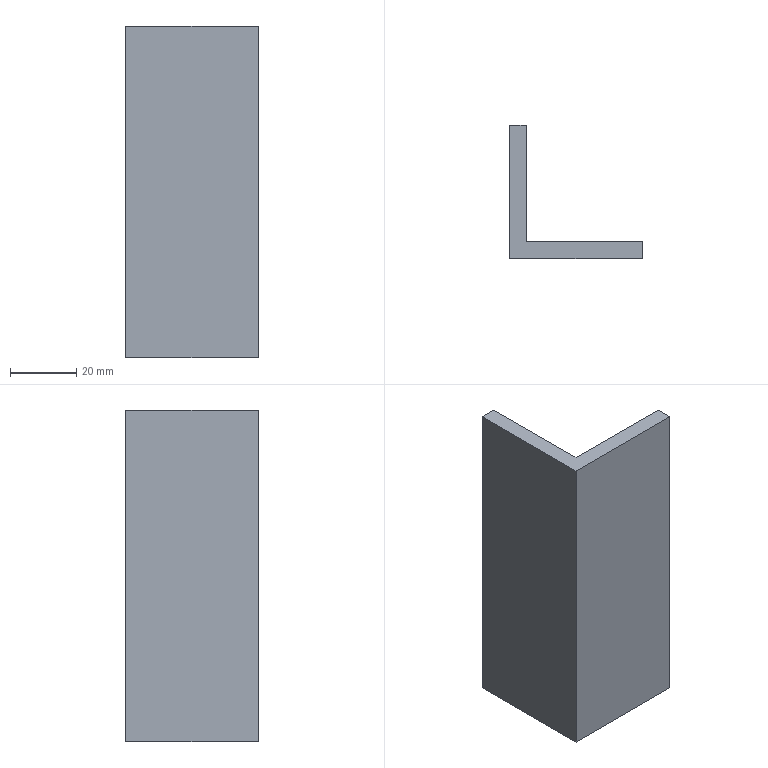Part | SolidWorks | features Extrusion 1 | 1 solid | 8 faces | box 40 x 40 x 100 mm | volume 37500 mm3 | plane 8
STEP:
#1=CARTESIAN_POINT('',(5.,0.,0.));
#2=VERTEX_POINT('',#1);
#3=CARTESIAN_POINT('',(0.,0.,0.));
#4=VERTEX_POINT('',#3);
#5=CARTESIAN_POINT('',(0.,0.,0.));
#6=DIRECTION('',(-1.,0.,0.));
#7=VECTOR('',#6,1000.);
#8=LINE('',#5,#7);
#9=EDGE_CURVE('',#2,#4,#8,.T.);
#10=ORIENTED_EDGE('',*,*,#9,.T.);
#11=CARTESIAN_POINT('',(0.,0.,100.));
#12=VERTEX_POINT('',#11);
#13=CARTESIAN_POINT('',(0.,0.,100.));
#14=DIRECTION('',(0.,0.,-1.));
#15=VECTOR('',#14,1000.);
#16=LINE('',#13,#15);
#17=EDGE_CURVE('',#12,#4,#16,.T.);
#18=ORIENTED_EDGE('',*,*,#17,.F.);
#19=CARTESIAN_POINT('',(5.,0.,100.));
#20=VERTEX_POINT('',#19);
#21=CARTESIAN_POINT('',(0.,0.,100.));
#22=DIRECTION('',(-1.,0.,0.));
#23=VECTOR('',#22,1000.);
#24=LINE('',#21,#23);
#25=EDGE_CURVE('',#20,#12,#24,.T.);
#26=ORIENTED_EDGE('',*,*,#25,.F.);
#27=CARTESIAN_POINT('',(5.,0.,100.));
#28=DIRECTION('',(0.,0.,-1.));
#29=VECTOR('',#28,1000.);
#30=LINE('',#27,#29);
#31=EDGE_CURVE('',#20,#2,#30,.T.);
#32=ORIENTED_EDGE('',*,*,#31,.T.);
#33=EDGE_LOOP('',(#10,#18,#26,#32));
#34=FACE_OUTER_BOUND('',#33,.T.);
#35=CARTESIAN_POINT('',(0.,0.,100.));
#36=DIRECTION('',(0.,-1.,0.));
#37=DIRECTION('',(0.,0.,-1.));
#38=AXIS2_PLACEMENT_3D('',#35,#36,#37);
#39=PLANE('',#38);
#40=ADVANCED_FACE('',(#34),#39,.F.);
#41=CARTESIAN_POINT('',(0.,-40.,0.));
#42=VERTEX_POINT('',#41);
#43=CARTESIAN_POINT('',(0.,0.,0.));
#44=DIRECTION('',(0.,-1.,0.));
#45=VECTOR('',#44,1000.);
#46=LINE('',#43,#45);
#47=EDGE_CURVE('',#4,#42,#46,.T.);
#48=ORIENTED_EDGE('',*,*,#47,.T.);
#49=CARTESIAN_POINT('',(0.,-40.,100.));
#50=VERTEX_POINT('',#49);
#51=CARTESIAN_POINT('',(0.,-40.,100.));
#52=DIRECTION('',(0.,0.,-1.));
#53=VECTOR('',#52,1000.);
#54=LINE('',#51,#53);
#55=EDGE_CURVE('',#50,#42,#54,.T.);
#56=ORIENTED_EDGE('',*,*,#55,.F.);
#57=CARTESIAN_POINT('',(0.,0.,100.));
#58=DIRECTION('',(0.,-1.,0.));
#59=VECTOR('',#58,1000.);
#60=LINE('',#57,#59);
#61=EDGE_CURVE('',#12,#50,#60,.T.);
#62=ORIENTED_EDGE('',*,*,#61,.F.);
#63=ORIENTED_EDGE('',*,*,#17,.T.);
#64=EDGE_LOOP('',(#48,#56,#62,#63));
#65=FACE_OUTER_BOUND('',#64,.T.);
#66=CARTESIAN_POINT('',(0.,0.,100.));
#67=DIRECTION('',(1.,0.,0.));
#68=DIRECTION('',(0.,1.,0.));
#69=AXIS2_PLACEMENT_3D('',#66,#67,#68);
#70=PLANE('',#69);
#71=ADVANCED_FACE('',(#65),#70,.F.);
#72=CARTESIAN_POINT('',(40.,-40.,0.));
#73=VERTEX_POINT('',#72);
#74=CARTESIAN_POINT('',(0.,-40.,0.));
#75=DIRECTION('',(1.,0.,0.));
#76=VECTOR('',#75,1000.);
#77=LINE('',#74,#76);
#78=EDGE_CURVE('',#42,#73,#77,.T.);
#79=ORIENTED_EDGE('',*,*,#78,.T.);
#80=CARTESIAN_POINT('',(40.,-40.,100.));
#81=VERTEX_POINT('',#80);
#82=CARTESIAN_POINT('',(40.,-40.,100.));
#83=DIRECTION('',(0.,0.,-1.));
#84=VECTOR('',#83,1000.);
#85=LINE('',#82,#84);
#86=EDGE_CURVE('',#81,#73,#85,.T.);
#87=ORIENTED_EDGE('',*,*,#86,.F.);
#88=CARTESIAN_POINT('',(0.,-40.,100.));
#89=DIRECTION('',(1.,0.,0.));
#90=VECTOR('',#89,1000.);
#91=LINE('',#88,#90);
#92=EDGE_CURVE('',#50,#81,#91,.T.);
#93=ORIENTED_EDGE('',*,*,#92,.F.);
#94=ORIENTED_EDGE('',*,*,#55,.T.);
#95=EDGE_LOOP('',(#79,#87,#93,#94));
#96=FACE_OUTER_BOUND('',#95,.T.);
#97=CARTESIAN_POINT('',(0.,-40.,100.));
#98=DIRECTION('',(0.,1.,0.));
#99=DIRECTION('',(0.,0.,1.));
#100=AXIS2_PLACEMENT_3D('',#97,#98,#99);
#101=PLANE('',#100);
#102=ADVANCED_FACE('',(#96),#101,.F.);
#103=CARTESIAN_POINT('',(40.,-35.,0.));
#104=VERTEX_POINT('',#103);
#105=CARTESIAN_POINT('',(40.,-40.,0.));
#106=DIRECTION('',(0.,1.,0.));
#107=VECTOR('',#106,1000.);
#108=LINE('',#105,#107);
#109=EDGE_CURVE('',#73,#104,#108,.T.);
#110=ORIENTED_EDGE('',*,*,#109,.T.);
#111=CARTESIAN_POINT('',(40.,-35.,100.));
#112=VERTEX_POINT('',#111);
#113=CARTESIAN_POINT('',(40.,-35.,100.));
#114=DIRECTION('',(0.,0.,-1.));
#115=VECTOR('',#114,1000.);
#116=LINE('',#113,#115);
#117=EDGE_CURVE('',#112,#104,#116,.T.);
#118=ORIENTED_EDGE('',*,*,#117,.F.);
#119=CARTESIAN_POINT('',(40.,-40.,100.));
#120=DIRECTION('',(0.,1.,0.));
#121=VECTOR('',#120,1000.);
#122=LINE('',#119,#121);
#123=EDGE_CURVE('',#81,#112,#122,.T.);
#124=ORIENTED_EDGE('',*,*,#123,.F.);
#125=ORIENTED_EDGE('',*,*,#86,.T.);
#126=EDGE_LOOP('',(#110,#118,#124,#125));
#127=FACE_OUTER_BOUND('',#126,.T.);
#128=CARTESIAN_POINT('',(40.,-40.,100.));
#129=DIRECTION('',(-1.,0.,0.));
#130=DIRECTION('',(0.,0.,1.));
#131=AXIS2_PLACEMENT_3D('',#128,#129,#130);
#132=PLANE('',#131);
#133=ADVANCED_FACE('',(#127),#132,.F.);
#134=CARTESIAN_POINT('',(5.,-35.,0.));
#135=VERTEX_POINT('',#134);
#136=CARTESIAN_POINT('',(5.,-35.,0.));
#137=DIRECTION('',(-1.,0.,0.));
#138=VECTOR('',#137,1000.);
#139=LINE('',#136,#138);
#140=EDGE_CURVE('',#104,#135,#139,.T.);
#141=ORIENTED_EDGE('',*,*,#140,.T.);
#142=CARTESIAN_POINT('',(5.,-35.,100.));
#143=VERTEX_POINT('',#142);
#144=CARTESIAN_POINT('',(5.,-35.,100.));
#145=DIRECTION('',(0.,0.,-1.));
#146=VECTOR('',#145,1000.);
#147=LINE('',#144,#146);
#148=EDGE_CURVE('',#143,#135,#147,.T.);
#149=ORIENTED_EDGE('',*,*,#148,.F.);
#150=CARTESIAN_POINT('',(5.,-35.,100.));
#151=DIRECTION('',(-1.,0.,0.));
#152=VECTOR('',#151,1000.);
#153=LINE('',#150,#152);
#154=EDGE_CURVE('',#112,#143,#153,.T.);
#155=ORIENTED_EDGE('',*,*,#154,.F.);
#156=ORIENTED_EDGE('',*,*,#117,.T.);
#157=EDGE_LOOP('',(#141,#149,#155,#156));
#158=FACE_OUTER_BOUND('',#157,.T.);
#159=CARTESIAN_POINT('',(5.,-35.,100.));
#160=DIRECTION('',(0.,-1.,0.));
#161=DIRECTION('',(0.,0.,-1.));
#162=AXIS2_PLACEMENT_3D('',#159,#160,#161);
#163=PLANE('',#162);
#164=ADVANCED_FACE('',(#158),#163,.F.);
#165=CARTESIAN_POINT('',(5.,0.,0.));
#166=DIRECTION('',(0.,1.,0.));
#167=VECTOR('',#166,1000.);
#168=LINE('',#165,#167);
#169=EDGE_CURVE('',#135,#2,#168,.T.);
#170=ORIENTED_EDGE('',*,*,#169,.T.);
#171=ORIENTED_EDGE('',*,*,#31,.F.);
#172=CARTESIAN_POINT('',(5.,0.,100.));
#173=DIRECTION('',(0.,1.,0.));
#174=VECTOR('',#173,1000.);
#175=LINE('',#172,#174);
#176=EDGE_CURVE('',#143,#20,#175,.T.);
#177=ORIENTED_EDGE('',*,*,#176,.F.);
#178=ORIENTED_EDGE('',*,*,#148,.T.);
#179=EDGE_LOOP('',(#170,#171,#177,#178));
#180=FACE_OUTER_BOUND('',#179,.T.);
#181=CARTESIAN_POINT('',(5.,0.,100.));
#182=DIRECTION('',(-1.,0.,0.));
#183=DIRECTION('',(0.,0.,1.));
#184=AXIS2_PLACEMENT_3D('',#181,#182,#183);
#185=PLANE('',#184);
#186=ADVANCED_FACE('',(#180),#185,.F.);
#187=ORIENTED_EDGE('',*,*,#25,.T.);
#188=ORIENTED_EDGE('',*,*,#61,.T.);
#189=ORIENTED_EDGE('',*,*,#92,.T.);
#190=ORIENTED_EDGE('',*,*,#123,.T.);
#191=ORIENTED_EDGE('',*,*,#154,.T.);
#192=ORIENTED_EDGE('',*,*,#176,.T.);
#193=EDGE_LOOP('',(#187,#188,#189,#190,#191,#192));
#194=FACE_OUTER_BOUND('',#193,.T.);
#195=CARTESIAN_POINT('',(0.,0.,100.));
#196=DIRECTION('',(0.,0.,-1.));
#197=DIRECTION('',(-1.,0.,0.));
#198=AXIS2_PLACEMENT_3D('',#195,#196,#197);
#199=PLANE('',#198);
#200=ADVANCED_FACE('',(#194),#199,.F.);
#201=ORIENTED_EDGE('',*,*,#9,.F.);
#202=ORIENTED_EDGE('',*,*,#169,.F.);
#203=ORIENTED_EDGE('',*,*,#140,.F.);
#204=ORIENTED_EDGE('',*,*,#109,.F.);
#205=ORIENTED_EDGE('',*,*,#78,.F.);
#206=ORIENTED_EDGE('',*,*,#47,.F.);
#207=EDGE_LOOP('',(#201,#202,#203,#204,#205,#206));
#208=FACE_OUTER_BOUND('',#207,.T.);
#209=CARTESIAN_POINT('',(0.,0.,0.));
#210=DIRECTION('',(0.,0.,-1.));
#211=DIRECTION('',(-1.,0.,0.));
#212=AXIS2_PLACEMENT_3D('',#209,#210,#211);
#213=PLANE('',#212);
#214=ADVANCED_FACE('',(#208),#213,.T.);
#215=CLOSED_SHELL('',(#40,#71,#102,#133,#164,#186,#200,#214));
#216=MANIFOLD_SOLID_BREP('',#215);
#217=CARTESIAN_POINT('',(0.,0.,0.));
#218=DIRECTION('',(0.,0.,1.));
#219=DIRECTION('',(1.,0.,0.));
#220=AXIS2_PLACEMENT_3D('',#217,#218,#219);
#221=(LENGTH_UNIT()NAMED_UNIT(*)SI_UNIT(.MILLI.,.METRE.));
#222=UNCERTAINTY_MEASURE_WITH_UNIT(LENGTH_MEASURE(0.00001),#221,'','');
#223=(NAMED_UNIT(*)PLANE_ANGLE_UNIT()SI_UNIT($,.RADIAN.));
#224=(NAMED_UNIT(*)SI_UNIT($,.STERADIAN.)SOLID_ANGLE_UNIT());
#225=(GEOMETRIC_REPRESENTATION_CONTEXT(3)GLOBAL_UNCERTAINTY_ASSIGNED_CONTEXT((#222))GLOBAL_UNIT_ASSIGNED_CONTEXT((#221,#223,#224))REPRESENTATION_CONTEXT('',''));
#226=ADVANCED_BREP_SHAPE_REPRESENTATION('',(#216,#220),#225);